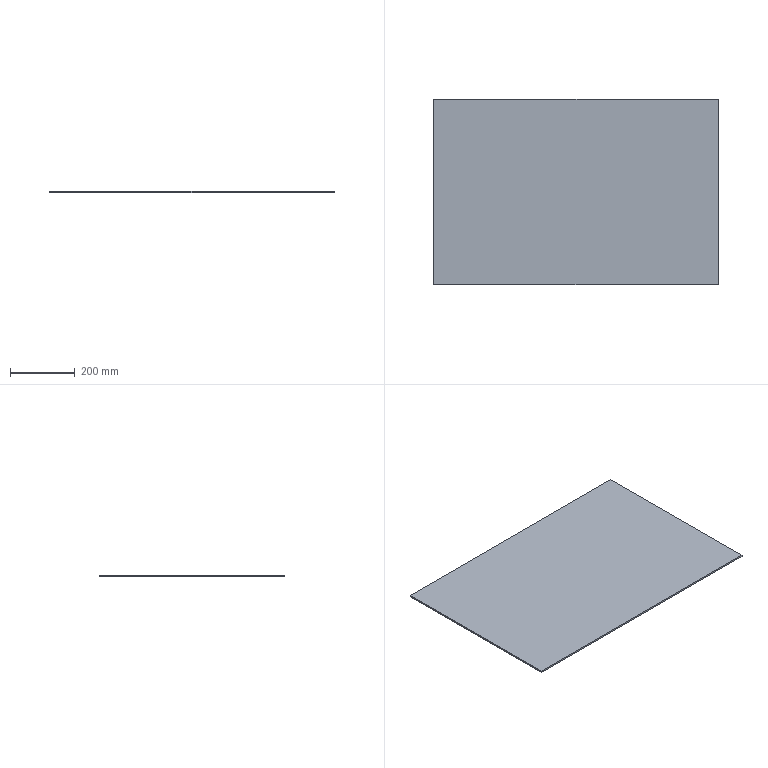Part | SolidWorks | features Extrusion 1, HoleWzd 1 | 1 solid | 6 faces | box 876 x 571 x 5 mm | volume 2500980 mm3 | plane 6
STEP:
#1=CARTESIAN_POINT('',(438.,-285.5,0.));
#2=VERTEX_POINT('',#1);
#3=CARTESIAN_POINT('',(438.,285.5,0.));
#4=VERTEX_POINT('',#3);
#5=CARTESIAN_POINT('',(438.,285.5,0.));
#6=DIRECTION('',(0.,1.,0.));
#7=VECTOR('',#6,1000.);
#8=LINE('',#5,#7);
#9=EDGE_CURVE('',#2,#4,#8,.T.);
#10=ORIENTED_EDGE('',*,*,#9,.T.);
#11=CARTESIAN_POINT('',(438.,285.5,5.));
#12=VERTEX_POINT('',#11);
#13=CARTESIAN_POINT('',(438.,285.5,5.));
#14=DIRECTION('',(0.,0.,-1.));
#15=VECTOR('',#14,1000.);
#16=LINE('',#13,#15);
#17=EDGE_CURVE('',#12,#4,#16,.T.);
#18=ORIENTED_EDGE('',*,*,#17,.F.);
#19=CARTESIAN_POINT('',(438.,-285.5,5.));
#20=VERTEX_POINT('',#19);
#21=CARTESIAN_POINT('',(438.,285.5,5.));
#22=DIRECTION('',(0.,1.,0.));
#23=VECTOR('',#22,1000.);
#24=LINE('',#21,#23);
#25=EDGE_CURVE('',#20,#12,#24,.T.);
#26=ORIENTED_EDGE('',*,*,#25,.F.);
#27=CARTESIAN_POINT('',(438.,-285.5,5.));
#28=DIRECTION('',(0.,0.,-1.));
#29=VECTOR('',#28,1000.);
#30=LINE('',#27,#29);
#31=EDGE_CURVE('',#20,#2,#30,.T.);
#32=ORIENTED_EDGE('',*,*,#31,.T.);
#33=EDGE_LOOP('',(#10,#18,#26,#32));
#34=FACE_OUTER_BOUND('',#33,.T.);
#35=CARTESIAN_POINT('',(438.,285.5,5.));
#36=DIRECTION('',(-1.,0.,0.));
#37=DIRECTION('',(0.,-1.,0.));
#38=AXIS2_PLACEMENT_3D('',#35,#36,#37);
#39=PLANE('',#38);
#40=ADVANCED_FACE('',(#34),#39,.F.);
#41=CARTESIAN_POINT('',(-438.,285.5,0.));
#42=VERTEX_POINT('',#41);
#43=CARTESIAN_POINT('',(-438.,285.5,0.));
#44=DIRECTION('',(-1.,0.,0.));
#45=VECTOR('',#44,1000.);
#46=LINE('',#43,#45);
#47=EDGE_CURVE('',#4,#42,#46,.T.);
#48=ORIENTED_EDGE('',*,*,#47,.T.);
#49=CARTESIAN_POINT('',(-438.,285.5,5.));
#50=VERTEX_POINT('',#49);
#51=CARTESIAN_POINT('',(-438.,285.5,5.));
#52=DIRECTION('',(0.,0.,-1.));
#53=VECTOR('',#52,1000.);
#54=LINE('',#51,#53);
#55=EDGE_CURVE('',#50,#42,#54,.T.);
#56=ORIENTED_EDGE('',*,*,#55,.F.);
#57=CARTESIAN_POINT('',(-438.,285.5,5.));
#58=DIRECTION('',(-1.,0.,0.));
#59=VECTOR('',#58,1000.);
#60=LINE('',#57,#59);
#61=EDGE_CURVE('',#12,#50,#60,.T.);
#62=ORIENTED_EDGE('',*,*,#61,.F.);
#63=ORIENTED_EDGE('',*,*,#17,.T.);
#64=EDGE_LOOP('',(#48,#56,#62,#63));
#65=FACE_OUTER_BOUND('',#64,.T.);
#66=CARTESIAN_POINT('',(-438.,285.5,5.));
#67=DIRECTION('',(0.,-1.,0.));
#68=DIRECTION('',(0.,0.,-1.));
#69=AXIS2_PLACEMENT_3D('',#66,#67,#68);
#70=PLANE('',#69);
#71=ADVANCED_FACE('',(#65),#70,.F.);
#72=CARTESIAN_POINT('',(-438.,-285.5,0.));
#73=VERTEX_POINT('',#72);
#74=CARTESIAN_POINT('',(-438.,285.5,0.));
#75=DIRECTION('',(0.,-1.,0.));
#76=VECTOR('',#75,1000.);
#77=LINE('',#74,#76);
#78=EDGE_CURVE('',#42,#73,#77,.T.);
#79=ORIENTED_EDGE('',*,*,#78,.T.);
#80=CARTESIAN_POINT('',(-438.,-285.5,5.));
#81=VERTEX_POINT('',#80);
#82=CARTESIAN_POINT('',(-438.,-285.5,5.));
#83=DIRECTION('',(0.,0.,-1.));
#84=VECTOR('',#83,1000.);
#85=LINE('',#82,#84);
#86=EDGE_CURVE('',#81,#73,#85,.T.);
#87=ORIENTED_EDGE('',*,*,#86,.F.);
#88=CARTESIAN_POINT('',(-438.,285.5,5.));
#89=DIRECTION('',(0.,-1.,0.));
#90=VECTOR('',#89,1000.);
#91=LINE('',#88,#90);
#92=EDGE_CURVE('',#50,#81,#91,.T.);
#93=ORIENTED_EDGE('',*,*,#92,.F.);
#94=ORIENTED_EDGE('',*,*,#55,.T.);
#95=EDGE_LOOP('',(#79,#87,#93,#94));
#96=FACE_OUTER_BOUND('',#95,.T.);
#97=CARTESIAN_POINT('',(-438.,285.5,5.));
#98=DIRECTION('',(1.,0.,0.));
#99=DIRECTION('',(0.,0.,-1.));
#100=AXIS2_PLACEMENT_3D('',#97,#98,#99);
#101=PLANE('',#100);
#102=ADVANCED_FACE('',(#96),#101,.F.);
#103=CARTESIAN_POINT('',(-438.,-285.5,0.));
#104=DIRECTION('',(1.,0.,0.));
#105=VECTOR('',#104,1000.);
#106=LINE('',#103,#105);
#107=EDGE_CURVE('',#73,#2,#106,.T.);
#108=ORIENTED_EDGE('',*,*,#107,.T.);
#109=ORIENTED_EDGE('',*,*,#31,.F.);
#110=CARTESIAN_POINT('',(-438.,-285.5,5.));
#111=DIRECTION('',(1.,0.,0.));
#112=VECTOR('',#111,1000.);
#113=LINE('',#110,#112);
#114=EDGE_CURVE('',#81,#20,#113,.T.);
#115=ORIENTED_EDGE('',*,*,#114,.F.);
#116=ORIENTED_EDGE('',*,*,#86,.T.);
#117=EDGE_LOOP('',(#108,#109,#115,#116));
#118=FACE_OUTER_BOUND('',#117,.T.);
#119=CARTESIAN_POINT('',(-438.,-285.5,5.));
#120=DIRECTION('',(0.,1.,0.));
#121=DIRECTION('',(0.,0.,1.));
#122=AXIS2_PLACEMENT_3D('',#119,#120,#121);
#123=PLANE('',#122);
#124=ADVANCED_FACE('',(#118),#123,.F.);
#125=ORIENTED_EDGE('',*,*,#25,.T.);
#126=ORIENTED_EDGE('',*,*,#61,.T.);
#127=ORIENTED_EDGE('',*,*,#92,.T.);
#128=ORIENTED_EDGE('',*,*,#114,.T.);
#129=EDGE_LOOP('',(#125,#126,#127,#128));
#130=FACE_OUTER_BOUND('',#129,.T.);
#131=CARTESIAN_POINT('',(0.,0.,5.));
#132=DIRECTION('',(0.,0.,1.));
#133=DIRECTION('',(1.,0.,0.));
#134=AXIS2_PLACEMENT_3D('',#131,#132,#133);
#135=PLANE('',#134);
#136=ADVANCED_FACE('',(#130),#135,.T.);
#137=ORIENTED_EDGE('',*,*,#9,.F.);
#138=ORIENTED_EDGE('',*,*,#107,.F.);
#139=ORIENTED_EDGE('',*,*,#78,.F.);
#140=ORIENTED_EDGE('',*,*,#47,.F.);
#141=EDGE_LOOP('',(#137,#138,#139,#140));
#142=FACE_OUTER_BOUND('',#141,.T.);
#143=CARTESIAN_POINT('',(0.,0.,0.));
#144=DIRECTION('',(0.,0.,1.));
#145=DIRECTION('',(1.,0.,0.));
#146=AXIS2_PLACEMENT_3D('',#143,#144,#145);
#147=PLANE('',#146);
#148=ADVANCED_FACE('',(#142),#147,.F.);
#149=CLOSED_SHELL('',(#40,#71,#102,#124,#136,#148));
#150=MANIFOLD_SOLID_BREP('',#149);
#151=CARTESIAN_POINT('',(0.,0.,0.));
#152=DIRECTION('',(0.,0.,1.));
#153=DIRECTION('',(1.,0.,0.));
#154=AXIS2_PLACEMENT_3D('',#151,#152,#153);
#155=(LENGTH_UNIT()NAMED_UNIT(*)SI_UNIT(.MILLI.,.METRE.));
#156=UNCERTAINTY_MEASURE_WITH_UNIT(LENGTH_MEASURE(0.00001),#155,'','');
#157=(NAMED_UNIT(*)PLANE_ANGLE_UNIT()SI_UNIT($,.RADIAN.));
#158=(NAMED_UNIT(*)SI_UNIT($,.STERADIAN.)SOLID_ANGLE_UNIT());
#159=(GEOMETRIC_REPRESENTATION_CONTEXT(3)GLOBAL_UNCERTAINTY_ASSIGNED_CONTEXT((#156))GLOBAL_UNIT_ASSIGNED_CONTEXT((#155,#157,#158))REPRESENTATION_CONTEXT('',''));
#160=ADVANCED_BREP_SHAPE_REPRESENTATION('',(#150,#154),#159);